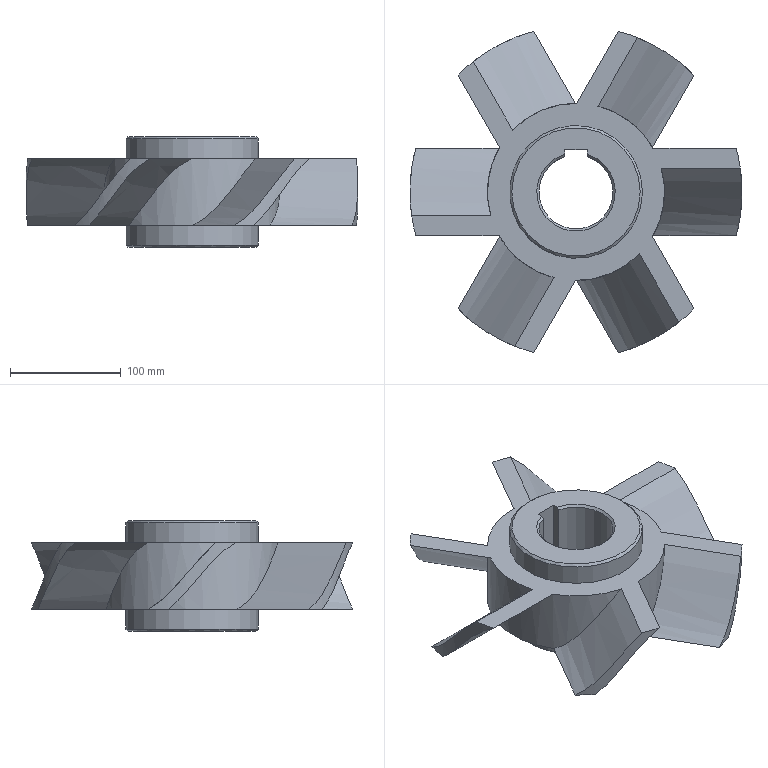Part | NX | features DATUM_CSYS 7, EXTRUDE 7, EXTRACT_BODY 6, SKETCH 6, BLEND 2, CHAMFER 1, Container 1, Geometry Instance 1, HOLE PACKAGE 1, SIMPLE HOLE 1, UNITE 1 | 1 solid | 38 faces | box 300.002 x 290.157 x 100 mm | volume 1656356 mm3 | cylinder 15 | spline 12 | plane 7 | cone 4 | commonest cylinder face diameters 160 x6 300 x6 120 x2 67 x1